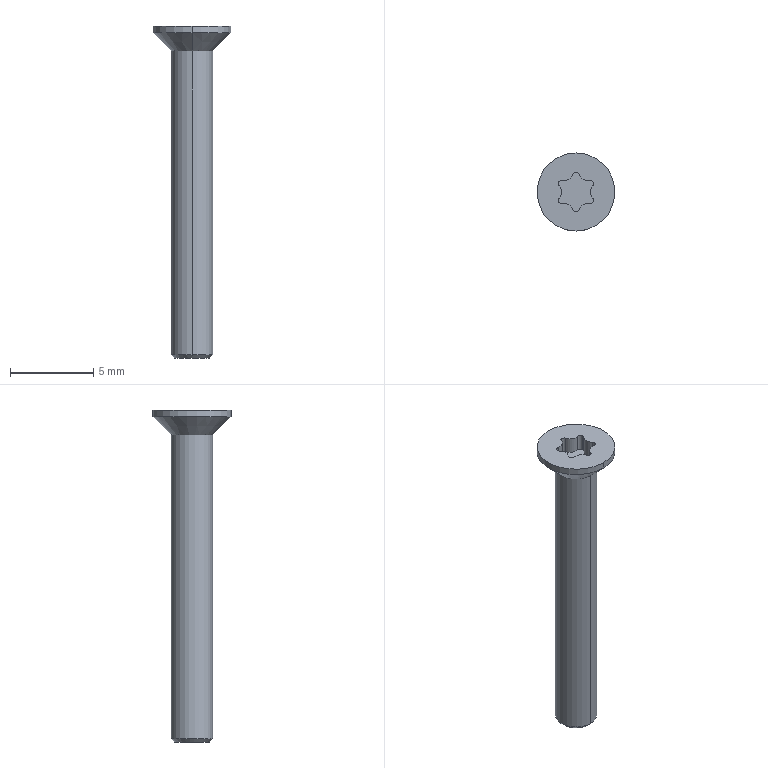Part | STEP file | ASND-0110-0219110005 | 1 solid | 26 faces | box 4.7 x 4.7 x 20 mm | volume 105.896 mm3 | cylinder 19 | cone 4 | plane 3 | commonest cylinder face diameters 0.4 x8 1.1 x7 2.5 x2 4.7 x2